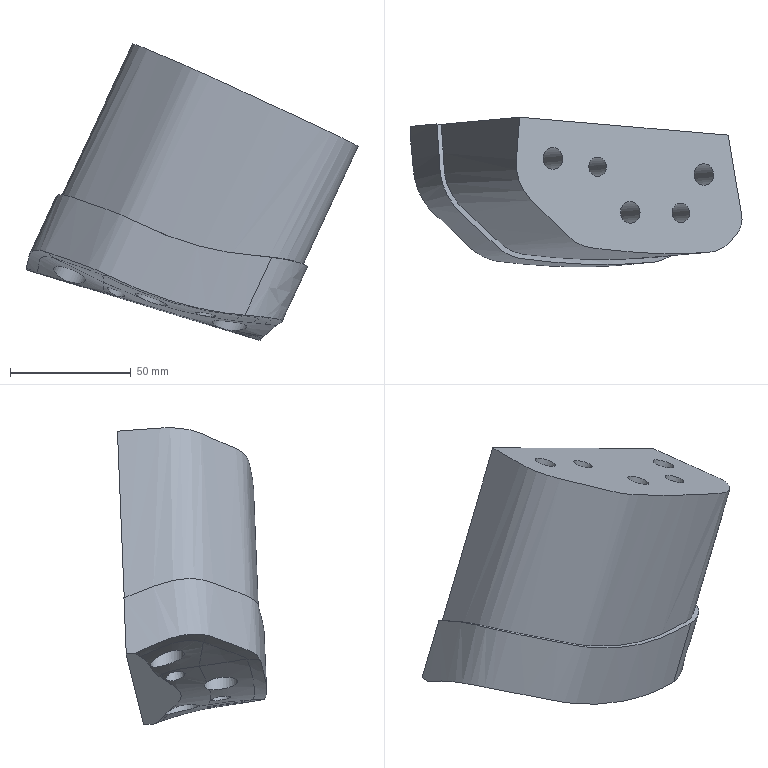Part | NX | features solid 2 | 1 solid | 34 faces | box 137.309 x 61.688 x 122.663 mm | volume 406441 mm3 | spline 20 | cylinder 8 | plane 6 | commonest cylinder face diameters 9 x3 14 x3 8 x2